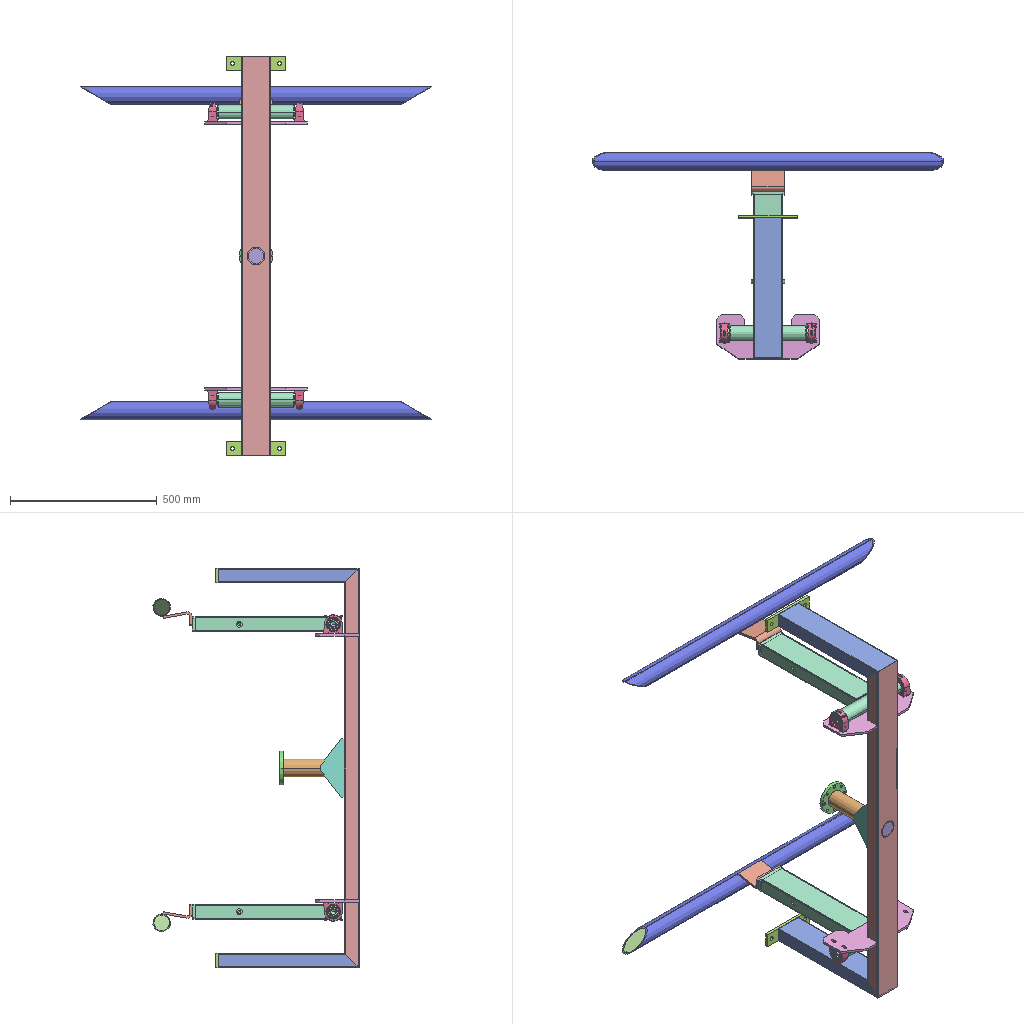Assembly | SolidWorks | 34 different items | 88 placed | box 1200 x 703 x 1364 mm
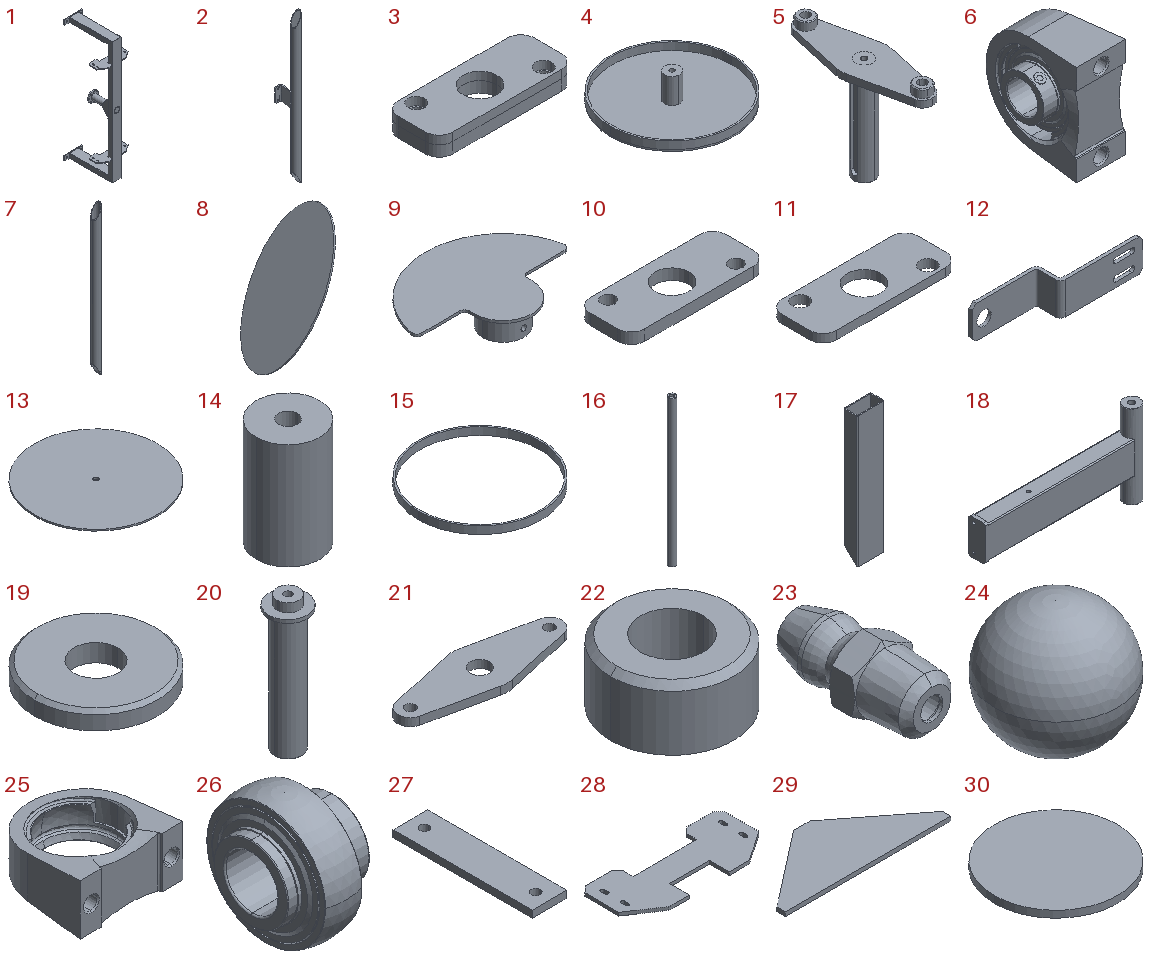Parts list (item | name | quantity | parent item | size | volume | features):
1 | (subassembly) | x1 | - | 350 x 490 x 1364 mm | 2989530 mm3 | -
2 | (subassembly) | x2 | - | 92.445 x 134.05 x 1200 mm | 757760 mm3 | features CompositeCurve 2
3 | (subassembly) | x1 | - | 50 x 20 x 7 mm | 5664 mm3 | -
4 | (subassembly) | x1 | - | 244.5 x 244.5 x 53 mm | 209212 mm3 | features CompositeCurve 1
5 | (subassembly) | x1 | - | 55 x 166 x 132 mm | 104297 mm3 | -
6 | (subassembly) | x4 | - | 34.3 x 65 x 65 mm | 66950 mm3 | features AEMSimFeature 1
7 | - | x2 | in 2 | 60.3 x 60.3 x 1200 mm | 628920 mm3 | features BaseBody 1, HoleWzd 1
8 | - | x4 | in 2 | 55.199 x 53.9 x 94.108 mm | 6846 mm3 | features ICE 4, Extrusion 1
9 | - | x1 | - | 93.161 x 65 x 15 mm | 10485 mm3 | features HoleWzd 3, Extrusion 1, Fillet 1, Revolution 1
10 | - | x1 | - | 50 x 20 x 4 mm | 3266 mm3 | features Extrusion 1
11 | - | x1 | - | 50 x 20 x 3 mm | 2398 mm3 | features Extrusion 1
12 | - | x1 | - | 185 x 34 x 40.884 mm | 31953 mm3 | features ICE 4, Fillet 2, Chamfer 1, Extrusion 1, HoleWzd 1
13 | - | x1 | - | 244.5 x 244.5 x 3 mm | 140663 mm3 | features Extrusion 1
14 | - | x1 | - | 30 x 30 x 50 mm | 32162 mm3 | features Extrusion 1
15 | - | x1 | - | 244.5 x 244.5 x 15 mm | 36387 mm3 | features Extrusion 1
16 | - | x1 | - | 20 x 20 x 415 mm | 96405 mm3 | features HoleWzd 2, Revolution 1
17 | - | x2 | in 1 | 100 x 50 x 480 mm | 389136 mm3 | features Extrusion 1, ICE 1
18 | - | x2 | - | 507 x 50 x 260 mm | 953629 mm3 | features HoleWzd 6, ICE 3, Chamfer 2, Revolution 2, Extrusion 1, Fillet 1
19 | - | x1 | - | 35 x 35 x 5 mm | 4143 mm3 | features Revolution 1
20 | - | x1 | - | 35 x 35 x 122 mm | 53457 mm3 | features ICE 3, HoleWzd 2, Chamfer 1, Extrusion 1
21 | - | x1 | - | 166 x 55 x 8 mm | 46251 mm3 | features Extrusion 1, HoleWzd 1, ICE 1
22 | - | x1 | - | 20 x 20 x 10 mm | 2294 mm3 | features Chamfer 1, Extrusion 1, HoleWzd 1
23 | - | x4 | in 6 | 7.001 x 16.4 x 8.083 mm | 360.824 mm3 | features BaseBody 1
24 | - | x32 | in 6 | 7.938 x 7.938 x 7.938 mm | 261.898 mm3 | features BaseBody 1
25 | - | x4 | in 6 | 65 x 65 x 32 mm | 47548 mm3 | features BaseBody 1
26 | - | x4 | in 6 | 31 x 47 x 47 mm | 16946 mm3 | features BaseBody 1
27 | - | x2 | in 1 | 50 x 200 x 10 mm | 97345 mm3 | features Extrusion 1
28 | - | x2 | in 1 | 350 x 150 x 8 mm | 290284 mm3 | features Extrusion 1
29 | - | x2 | in 1 | 200 x 80 x 5 mm | 48500 mm3 | features Extrusion 1
30 | - | x1 | in 1 | 53.9 x 53.9 x 3 mm | 6845 mm3 | features Extrusion 1
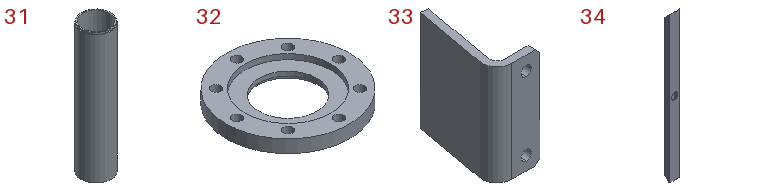31 | - | x1 | in 1 | 60.3 x 60.3 x 261 mm | 149181 mm3 | features Extrusion 1, ICE 1, Shell 1
32 | - | x1 | in 1 | 115 x 115 x 12 mm | 76316 mm3 | features ICE 4, Extrusion 1
33 | - | x2 | in 2 | 46.932 x 98.481 x 110 mm | 115150 mm3 | features Fillet 2, Chamfer 1, Extrusion 1, HoleWzd 1, ICE 1
34 | - | x1 | in 1 | 100 x 50 x 1364 mm | 1106656 mm3 | features ICE 2, Extrusion 1
Mates (type | each side: item.copy, entity, surface, feature):
In the top assembly
Coincident | 28.1 face plane Boss-Extrude 1 | 25.1 face plane SYF 504 -h(1)
Coincident | 28.2 face plane Boss-Extrude 1 | 25.2 face plane SYF 504 -h(1)
Slot | 25.2 face cylinder SYF 504 -h(1) | 28.2 face plane Boss-Extrude 1 | 2 times
Slot | 25.1 face cylinder SYF 504 -h(1) | 28.1 face plane Boss-Extrude 1 | 2 times
Concentric | 26.1 face cylinder YAR 204-2F-28.210300220447-b(1) | 18.1 face cylinder Revolve 2
Parallel | 27.1 face plane Boss-Extrude 1 | 18.1 face plane Boss-Extrude 1
Coincident | 18.1 face plane Boss-Extrude 1 | 18.2 face plane Boss-Extrude 1
Coincident | 18.1 face plane Cut-Extrude 1 | 18.2 face plane Cut-Extrude 1
Concentric | 26.2 edge | 18.2 face cylinder M20 Tapped Hole 2
Concentric | 18.1 face cylinder Revolve 2 | 26.3 face cylinder YAR 204-2F-28.210300220447-b(1)
Coincident | 28.2 face plane Boss-Extrude 1 | 25.3 face plane SYF 504 -h(1)
Slot | 28.2 face plane Boss-Extrude 1 | 25.3 face cylinder SYF 504 -h(1)
Slot | 25.3 face cylinder SYF 504 -h(1) | 28.2 face plane Boss-Extrude 1
Coincident | 28.1 face plane Boss-Extrude 1 | 25.4 face plane SYF 504 -h(1)
Slot | 25.4 face cylinder SYF 504 -h(1) | 28.1 face plane Boss-Extrude 1
Slot | 28.1 face plane Boss-Extrude 1 | 25.4 face cylinder SYF 504 -h(1)
Width | 18.2 face plane Cut-Extrude 1 | 18.2 face plane Cut-Extrude 2 | 25.1 face plane SYF 504 -h(1) | 25.4 face plane SYF 504 -h(1)
Coincident | 18.2 face plane Boss-Extrude 1 | 33.1 face plane Boss-Extrude 1
Concentric | 18.2 edge | 33.1 edge
Concentric | 18.2 face cylinder Ø8.5 (8.5) DiameterHole 1 | 33.1 face cylinder Ø11.0 (11) DiameterHole 1
Coincident | 18.1 face plane Boss-Extrude 1 | 33.2 face plane Boss-Extrude 1
Concentric | 18.1 edge | 33.2 edge | 2 times
Concentric | 32.1 face cylinder Boss-Extrude 1 | 19.1 face cylinder Revolve 1
Coincident | 32.1 face plane Cut-Extrude 1 | 19.1 face plane Revolve 1
In subassembly 2
Coincident | 7.1 face plane Input 3 | 8.1 face plane Cut-Extrude 4
Coincident | 7.1 face plane Input 3 | 8.2 face plane Cut-Extrude 4
Tangent | 33.3 face plane Boss-Extrude 1 | 7.1 face cylinder Input 3
DistanceDim | 33.3 face plane Boss-Extrude 1 | 7.1 face cylinder Input 3
Coincident | 7.1 plane | 8.1 plane | 2 times
Perpendicular | 7.1 plane | 8.2 plane | 2 times
Coincident | 8.1 plane | 8.2 plane | 2 times
Parallel | 33.3 face plane Boss-Extrude 1 | 2.1 plane
Width | 8.2 face plane Cut-Extrude 4 | 8.1 face plane Cut-Extrude 4 | 33.3 face plane Boss-Extrude 1 | 33.3 face plane Boss-Extrude 1
In subassembly 1
Coincident | 34.1 face plane Cut-Extrude 1 | 17.1 face plane Cut-Extrude 1
Coincident | 34.1 face plane Boss-Extrude 1 | 17.1 face plane Boss-Extrude 1
Coincident | 34.1 edge | 17.1 edge
Coincident | 34.1 face plane Cut-Extrude 1 | 17.2 face plane Cut-Extrude 1
Coincident | 34.1 face plane Boss-Extrude 1 | 17.2 face plane Boss-Extrude 1
Coincident | 34.1 edge | 17.2 edge
Coincident | 17.1 face plane Boss-Extrude 1 | 27.2 face plane Boss-Extrude 1
Width | 17.1 face plane Boss-Extrude 1 | 17.1 face plane Boss-Extrude 1 | 27.2 face plane Boss-Extrude 1 | 27.2 face plane Boss-Extrude 1
Width | 27.2 face plane Boss-Extrude 1 | 27.2 face plane Boss-Extrude 1 | 17.1 face plane Boss-Extrude 1 | 17.1 face plane Boss-Extrude 1
Coincident | 27.2 face plane Boss-Extrude 1 | 27.3 face plane Boss-Extrude 1 | 2 times
Width | 27.3 face plane Boss-Extrude 1 | 27.3 face plane Boss-Extrude 1 | 17.2 face plane Boss-Extrude 1 | 17.2 face plane Boss-Extrude 1
Coincident | 34.1 face plane Boss-Extrude 1 | 28.3 face plane Boss-Extrude 1 | 2 times
Coincident | 28.3 face plane Boss-Extrude 1 | 28.4 face plane Boss-Extrude 1 | 2 times
DistanceDim | 28.3 face plane Boss-Extrude 1 | 28.4 face plane Boss-Extrude 1
DistanceDim | 28.3 face plane Boss-Extrude 1 | 17.1 face plane Boss-Extrude 1
Concentric | 34.1 face cylinder Cut-Extrude 2 | 31.1 face cylinder Boss-Extrude 1
Coincident | 34.1 face plane Boss-Extrude 1 | 31.1 face plane Boss-Extrude 1
Concentric | 31.1 face cylinder Shell 1 | 30.1 face cylinder Boss-Extrude 1
Coincident | 34.1 face plane Boss-Extrude 1 | 30.1 face plane Boss-Extrude 1
Parallel | 34.1 face plane Boss-Extrude 1 | 29.1 face plane Boss-Extrude 1
Coincident | 34.1 face plane Boss-Extrude 1 | 29.1 face plane Boss-Extrude 1
Width | 28.3 face plane Boss-Extrude 1 | 28.4 face plane Boss-Extrude 1 | 29.1 face plane Boss-Extrude 1 | 29.1 face plane Boss-Extrude 1
Tangent | 29.1 face plane Boss-Extrude 1 | 31.1 face cylinder Boss-Extrude 1
Coincident | 29.1 face plane Boss-Extrude 1 | 29.2 face plane Boss-Extrude 1 | 2 times
Tangent | 31.1 face cylinder Boss-Extrude 1 | 29.2 face plane Boss-Extrude 1
Concentric | 31.1 face cylinder Boss-Extrude 1 | 32.2 face cylinder Boss-Extrude 1
Coincident | 31.1 face plane Cut-Extrude 1 | 32.2 face plane Boss-Extrude 1
Coincident | 31.1 plane | 32.2 plane
Parallel | 34.1 plane | 31.1 plane